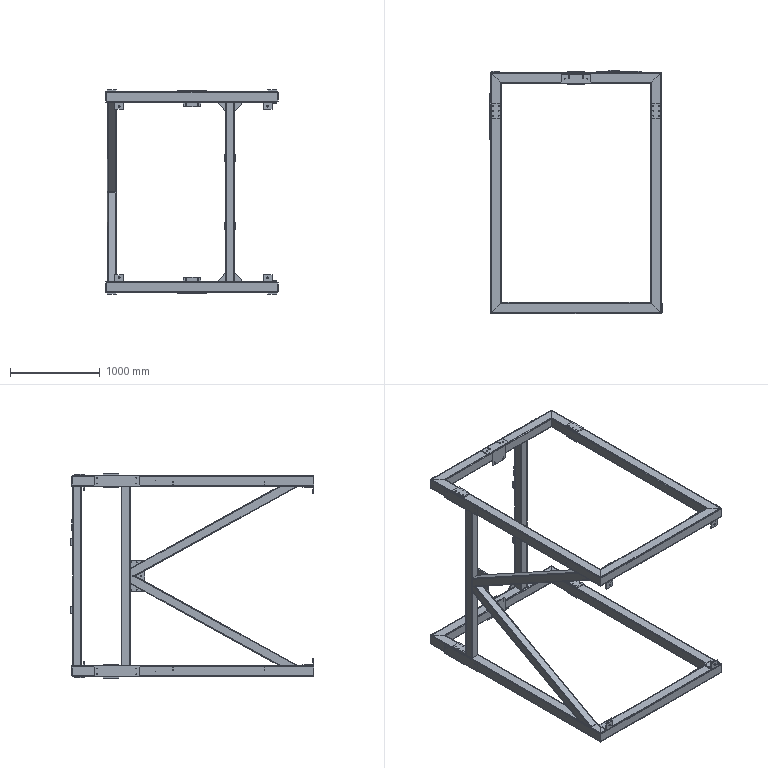Part | SolidWorks | features CompositeCurve 25 | 50 solids | 1095 faces | box 1920 x 2705 x 2270 mm | volume 51706109 mm3 | cylinder 722 | plane 373 | commonest cylinder face diameters 10.2 x202 15 x148 6.8 x68 5 x56 10 x48 20 x48